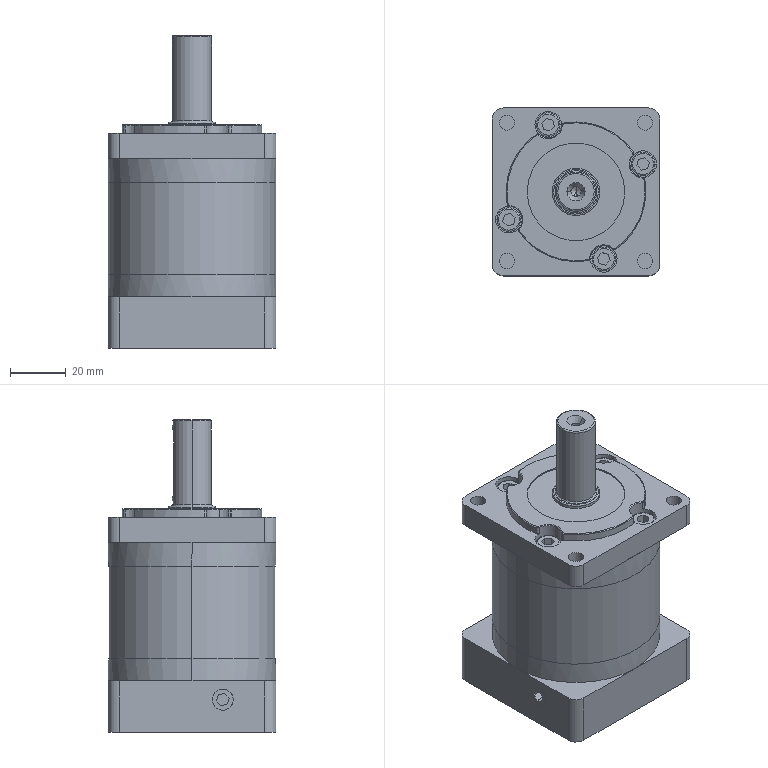Part | SolidWorks | features BaseBody 3 | 3 solids | 301 faces | box 60 x 60 x 112 mm | volume 219786 mm3 | plane 129 | cylinder 119 | cone 31 | spline 22 | commonest cylinder face diameters 4 x10 50 x10 2 x9 3.3 x8 5.5 x8 7 x8